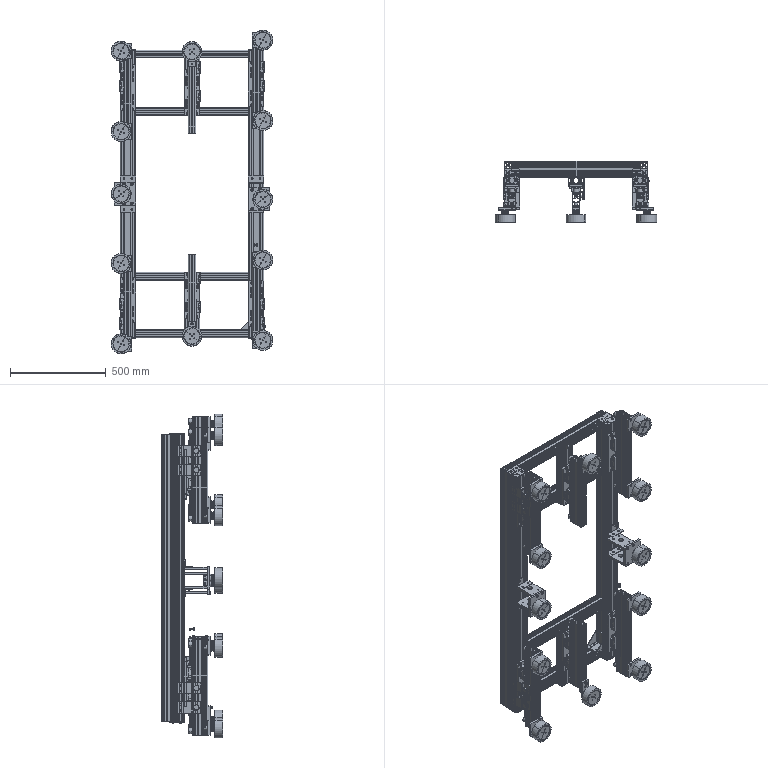Part | SolidWorks | 180 solids | 12106 faces | volume 18985349 mm3 | plane 7529 | cylinder 2564 | spline 1162 | cone 810 | torus 28 | sphere 13 | commonest cylinder face diameters 9 x256 1 x244 6 x204 6.4 x192 2 x132 4.2 x96